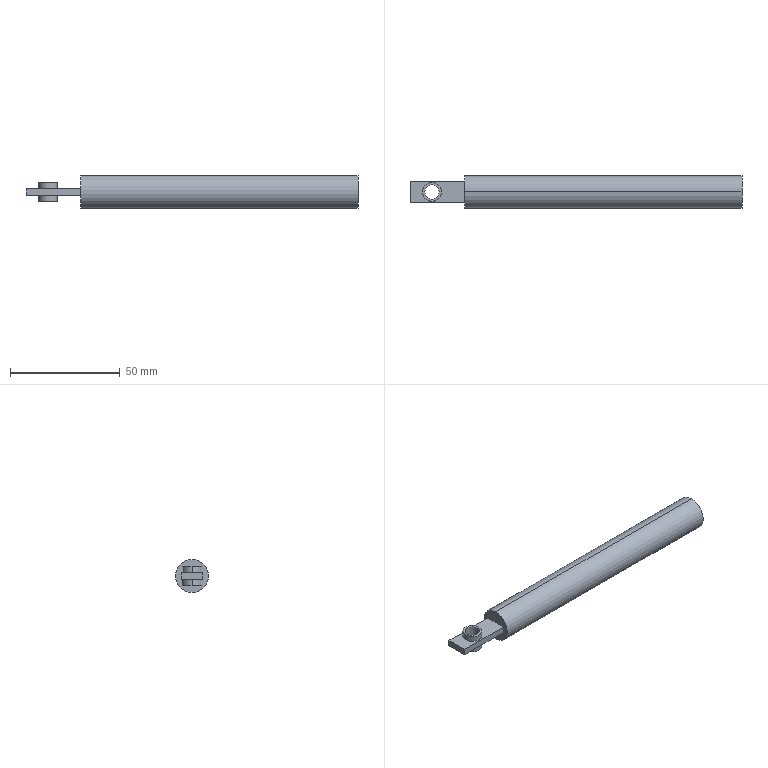Part | STEP file | Gas spring FGS 15089-100 body | 1 solid | 20 faces | box 151 x 15 x 15 mm | volume 18389 mm3 | cylinder 10 | plane 10 | commonest cylinder face diameters 8.5 x4 6.5 x2 7 x2 15 x2
STEP:
#1=CARTESIAN_POINT('',(0.,0.,0.));
#2=DIRECTION('',(0.,0.,1.));
#3=DIRECTION('',(1.,0.,0.));
#4=AXIS2_PLACEMENT_3D('',#1,#2,#3);
#5=CARTESIAN_POINT('',(-11.75,0.,-4.25));
#6=VERTEX_POINT('',#5);
#7=CARTESIAN_POINT('',(-11.75,0.,4.25));
#8=VERTEX_POINT('',#7);
#9=CARTESIAN_POINT('',(-11.75,0.,-4.25));
#10=DIRECTION('',(0.,0.,1.));
#11=VECTOR('',#10,1.);
#12=LINE('',#9,#11);
#13=CARTESIAN_POINT('',(-15.,0.,-4.25));
#14=DIRECTION('',(0.,0.,1.));
#15=DIRECTION('',(1.,0.,0.));
#16=AXIS2_PLACEMENT_3D('',#13,#14,#15);
#17=CYLINDRICAL_SURFACE('',#16,3.25);
#18=CARTESIAN_POINT('',(6.283,0.));
#19=DIRECTION('',(0.,1.));
#20=VECTOR('',#19,1.);
#21=LINE('',#18,#20);
#22=(GEOMETRIC_REPRESENTATION_CONTEXT(2)PARAMETRIC_REPRESENTATION_CONTEXT()REPRESENTATION_CONTEXT('',''));
#23=DEFINITIONAL_REPRESENTATION('',(#21),#22);
#24=PCURVE('',#17,#23);
#25=CARTESIAN_POINT('',(-15.,0.,-4.25));
#26=DIRECTION('',(0.,0.,1.));
#27=DIRECTION('',(1.,0.,0.));
#28=AXIS2_PLACEMENT_3D('',#25,#26,#27);
#29=CYLINDRICAL_SURFACE('',#28,3.25);
#30=CARTESIAN_POINT('',(0.,0.));
#31=DIRECTION('',(0.,1.));
#32=VECTOR('',#31,1.);
#33=LINE('',#30,#32);
#34=(GEOMETRIC_REPRESENTATION_CONTEXT(2)PARAMETRIC_REPRESENTATION_CONTEXT()REPRESENTATION_CONTEXT('',''));
#35=DEFINITIONAL_REPRESENTATION('',(#33),#34);
#36=PCURVE('',#29,#35);
#37=SURFACE_CURVE('',#12,(#24,#36),.PCURVE_S1.);
#38=EDGE_CURVE('',#6,#8,#37,.T.);
#39=ORIENTED_EDGE('',*,*,#38,.T.);
#40=CARTESIAN_POINT('',(-18.25,0.,4.25));
#41=VERTEX_POINT('',#40);
#42=CARTESIAN_POINT('',(-15.,0.,4.25));
#43=DIRECTION('',(0.,0.,1.));
#44=DIRECTION('',(1.,0.,0.));
#45=AXIS2_PLACEMENT_3D('',#42,#43,#44);
#46=CIRCLE('',#45,3.25);
#47=CARTESIAN_POINT('',(0.,8.5));
#48=DIRECTION('',(1.,0.));
#49=VECTOR('',#48,1.);
#50=LINE('',#47,#49);
#51=(GEOMETRIC_REPRESENTATION_CONTEXT(2)PARAMETRIC_REPRESENTATION_CONTEXT()REPRESENTATION_CONTEXT('',''));
#52=DEFINITIONAL_REPRESENTATION('',(#50),#51);
#53=PCURVE('',#17,#52);
#54=CARTESIAN_POINT('',(-19.301,-4.301,4.25));
#55=DIRECTION('',(0.,0.,1.));
#56=DIRECTION('',(1.,0.,0.));
#57=AXIS2_PLACEMENT_3D('',#54,#55,#56);
#58=PLANE('',#57);
#59=CARTESIAN_POINT('',(4.301,4.301));
#60=DIRECTION('',(1.,0.));
#61=AXIS2_PLACEMENT_2D('',#59,#60);
#62=CIRCLE('',#61,3.25);
#63=(GEOMETRIC_REPRESENTATION_CONTEXT(2)PARAMETRIC_REPRESENTATION_CONTEXT()REPRESENTATION_CONTEXT('',''));
#64=DEFINITIONAL_REPRESENTATION('',(#62),#63);
#65=PCURVE('',#58,#64);
#66=SURFACE_CURVE('',#46,(#53,#65),.PCURVE_S1.);
#67=EDGE_CURVE('',#41,#8,#66,.T.);
#68=ORIENTED_EDGE('',*,*,#67,.F.);
#69=CARTESIAN_POINT('',(-18.25,0.,-4.25));
#70=VERTEX_POINT('',#69);
#71=CARTESIAN_POINT('',(-18.25,0.,-4.25));
#72=DIRECTION('',(0.,0.,1.));
#73=VECTOR('',#72,1.);
#74=LINE('',#71,#73);
#75=CARTESIAN_POINT('',(3.142,0.));
#76=DIRECTION('',(0.,1.));
#77=VECTOR('',#76,1.);
#78=LINE('',#75,#77);
#79=(GEOMETRIC_REPRESENTATION_CONTEXT(2)PARAMETRIC_REPRESENTATION_CONTEXT()REPRESENTATION_CONTEXT('',''));
#80=DEFINITIONAL_REPRESENTATION('',(#78),#79);
#81=PCURVE('',#17,#80);
#82=CARTESIAN_POINT('',(3.142,0.));
#83=DIRECTION('',(0.,1.));
#84=VECTOR('',#83,1.);
#85=LINE('',#82,#84);
#86=(GEOMETRIC_REPRESENTATION_CONTEXT(2)PARAMETRIC_REPRESENTATION_CONTEXT()REPRESENTATION_CONTEXT('',''));
#87=DEFINITIONAL_REPRESENTATION('',(#85),#86);
#88=PCURVE('',#29,#87);
#89=SURFACE_CURVE('',#74,(#81,#88),.PCURVE_S1.);
#90=EDGE_CURVE('',#70,#41,#89,.T.);
#91=ORIENTED_EDGE('',*,*,#90,.F.);
#92=CARTESIAN_POINT('',(-15.,0.,-4.25));
#93=DIRECTION('',(0.,0.,-1.));
#94=DIRECTION('',(1.,0.,0.));
#95=AXIS2_PLACEMENT_3D('',#92,#93,#94);
#96=CIRCLE('',#95,3.25);
#97=CARTESIAN_POINT('',(6.283,0.));
#98=DIRECTION('',(-1.,0.));
#99=VECTOR('',#98,1.);
#100=LINE('',#97,#99);
#101=(GEOMETRIC_REPRESENTATION_CONTEXT(2)PARAMETRIC_REPRESENTATION_CONTEXT()REPRESENTATION_CONTEXT('',''));
#102=DEFINITIONAL_REPRESENTATION('',(#100),#101);
#103=PCURVE('',#17,#102);
#104=CARTESIAN_POINT('',(-19.301,-4.301,-4.25));
#105=DIRECTION('',(0.,0.,1.));
#106=DIRECTION('',(1.,0.,0.));
#107=AXIS2_PLACEMENT_3D('',#104,#105,#106);
#108=PLANE('',#107);
#109=CARTESIAN_POINT('',(7.551,4.301));
#110=CARTESIAN_POINT('',(7.551,-1.328));
#111=CARTESIAN_POINT('',(2.676,1.486));
#112=CARTESIAN_POINT('',(-2.199,4.301));
#113=CARTESIAN_POINT('',(2.676,7.116));
#114=CARTESIAN_POINT('',(7.551,9.93));
#115=CARTESIAN_POINT('',(7.551,4.301));
#116=(BOUNDED_CURVE()B_SPLINE_CURVE(2,(#109,#110,#111,#112,#113,#114,#115),.UNSPECIFIED.,.T.,.F.)B_SPLINE_CURVE_WITH_KNOTS((1,2,2,2,2,1),(-2.094,0.,2.094,4.189,6.283,8.378),.UNSPECIFIED.)CURVE()GEOMETRIC_REPRESENTATION_ITEM()RATIONAL_B_SPLINE_CURVE((1.,0.5,1.,0.5,1.,0.5,1.))REPRESENTATION_ITEM(''));
#117=(GEOMETRIC_REPRESENTATION_CONTEXT(2)PARAMETRIC_REPRESENTATION_CONTEXT()REPRESENTATION_CONTEXT('',''));
#118=DEFINITIONAL_REPRESENTATION('',(#116),#117);
#119=PCURVE('',#108,#118);
#120=SURFACE_CURVE('',#96,(#103,#119),.PCURVE_S1.);
#121=EDGE_CURVE('',#6,#70,#120,.T.);
#122=ORIENTED_EDGE('',*,*,#121,.F.);
#123=EDGE_LOOP('',(#39,#68,#91,#122));
#124=FACE_BOUND('',#123,.F.);
#125=ADVANCED_FACE('',(#124),#17,.F.);
#126=CARTESIAN_POINT('',(-10.75,0.,4.25));
#127=VERTEX_POINT('',#126);
#128=CARTESIAN_POINT('',(-19.25,0.,4.25));
#129=VERTEX_POINT('',#128);
#130=CARTESIAN_POINT('',(-15.,0.,4.25));
#131=DIRECTION('',(0.,0.,1.));
#132=DIRECTION('',(-1.,0.,0.));
#133=AXIS2_PLACEMENT_3D('',#130,#131,#132);
#134=CIRCLE('',#133,4.25);
#135=CARTESIAN_POINT('',(-15.,0.,4.25));
#136=DIRECTION('',(0.,0.,-1.));
#137=DIRECTION('',(-1.,0.,0.));
#138=AXIS2_PLACEMENT_3D('',#135,#136,#137);
#139=CYLINDRICAL_SURFACE('',#138,4.25);
#140=CARTESIAN_POINT('',(6.283,0.));
#141=DIRECTION('',(-1.,0.));
#142=VECTOR('',#141,1.);
#143=LINE('',#140,#142);
#144=(GEOMETRIC_REPRESENTATION_CONTEXT(2)PARAMETRIC_REPRESENTATION_CONTEXT()REPRESENTATION_CONTEXT('',''));
#145=DEFINITIONAL_REPRESENTATION('',(#143),#144);
#146=PCURVE('',#139,#145);
#147=CARTESIAN_POINT('',(4.301,4.301));
#148=DIRECTION('',(-1.,0.));
#149=AXIS2_PLACEMENT_2D('',#147,#148);
#150=CIRCLE('',#149,4.25);
#151=(GEOMETRIC_REPRESENTATION_CONTEXT(2)PARAMETRIC_REPRESENTATION_CONTEXT()REPRESENTATION_CONTEXT('',''));
#152=DEFINITIONAL_REPRESENTATION('',(#150),#151);
#153=PCURVE('',#58,#152);
#154=SURFACE_CURVE('',#134,(#146,#153),.PCURVE_S1.);
#155=EDGE_CURVE('',#127,#129,#154,.T.);
#156=ORIENTED_EDGE('',*,*,#155,.F.);
#157=CARTESIAN_POINT('',(-10.75,0.,1.5));
#158=VERTEX_POINT('',#157);
#159=CARTESIAN_POINT('',(-10.75,0.,4.25));
#160=DIRECTION('',(0.,0.,-1.));
#161=VECTOR('',#160,1.);
#162=LINE('',#159,#161);
#163=CARTESIAN_POINT('',(3.142,0.));
#164=DIRECTION('',(0.,1.));
#165=VECTOR('',#164,1.);
#166=LINE('',#163,#165);
#167=(GEOMETRIC_REPRESENTATION_CONTEXT(2)PARAMETRIC_REPRESENTATION_CONTEXT()REPRESENTATION_CONTEXT('',''));
#168=DEFINITIONAL_REPRESENTATION('',(#166),#167);
#169=PCURVE('',#139,#168);
#170=CARTESIAN_POINT('',(-15.,0.,4.25));
#171=DIRECTION('',(0.,0.,-1.));
#172=DIRECTION('',(-1.,0.,0.));
#173=AXIS2_PLACEMENT_3D('',#170,#171,#172);
#174=CYLINDRICAL_SURFACE('',#173,4.25);
#175=CARTESIAN_POINT('',(3.142,0.));
#176=DIRECTION('',(0.,1.));
#177=VECTOR('',#176,1.);
#178=LINE('',#175,#177);
#179=(GEOMETRIC_REPRESENTATION_CONTEXT(2)PARAMETRIC_REPRESENTATION_CONTEXT()REPRESENTATION_CONTEXT('',''));
#180=DEFINITIONAL_REPRESENTATION('',(#178),#179);
#181=PCURVE('',#174,#180);
#182=SURFACE_CURVE('',#162,(#169,#181),.PCURVE_S1.);
#183=EDGE_CURVE('',#127,#158,#182,.T.);
#184=ORIENTED_EDGE('',*,*,#183,.T.);
#185=CARTESIAN_POINT('',(-19.25,0.,1.5));
#186=VERTEX_POINT('',#185);
#187=CARTESIAN_POINT('',(-15.,0.,1.5));
#188=DIRECTION('',(0.,0.,-1.));
#189=DIRECTION('',(-1.,0.,0.));
#190=AXIS2_PLACEMENT_3D('',#187,#188,#189);
#191=CIRCLE('',#190,4.25);
#192=CARTESIAN_POINT('',(0.,2.75));
#193=DIRECTION('',(1.,0.));
#194=VECTOR('',#193,1.);
#195=LINE('',#192,#194);
#196=(GEOMETRIC_REPRESENTATION_CONTEXT(2)PARAMETRIC_REPRESENTATION_CONTEXT()REPRESENTATION_CONTEXT('',''));
#197=DEFINITIONAL_REPRESENTATION('',(#195),#196);
#198=PCURVE('',#139,#197);
#199=CARTESIAN_POINT('',(0.,-5.,1.5));
#200=DIRECTION('',(0.,0.,-1.));
#201=DIRECTION('',(-1.,0.,0.));
#202=AXIS2_PLACEMENT_3D('',#199,#200,#201);
#203=PLANE('',#202);
#204=CARTESIAN_POINT('',(15.,5.));
#205=DIRECTION('',(1.,0.));
#206=AXIS2_PLACEMENT_2D('',#204,#205);
#207=CIRCLE('',#206,4.25);
#208=(GEOMETRIC_REPRESENTATION_CONTEXT(2)PARAMETRIC_REPRESENTATION_CONTEXT()REPRESENTATION_CONTEXT('',''));
#209=DEFINITIONAL_REPRESENTATION('',(#207),#208);
#210=PCURVE('',#203,#209);
#211=SURFACE_CURVE('',#191,(#198,#210),.PCURVE_S1.);
#212=EDGE_CURVE('',#186,#158,#211,.T.);
#213=ORIENTED_EDGE('',*,*,#212,.F.);
#214=CARTESIAN_POINT('',(-19.25,0.,4.25));
#215=DIRECTION('',(0.,0.,-1.));
#216=VECTOR('',#215,1.);
#217=LINE('',#214,#216);
#218=CARTESIAN_POINT('',(0.,0.));
#219=DIRECTION('',(0.,1.));
#220=VECTOR('',#219,1.);
#221=LINE('',#218,#220);
#222=(GEOMETRIC_REPRESENTATION_CONTEXT(2)PARAMETRIC_REPRESENTATION_CONTEXT()REPRESENTATION_CONTEXT('',''));
#223=DEFINITIONAL_REPRESENTATION('',(#221),#222);
#224=PCURVE('',#139,#223);
#225=CARTESIAN_POINT('',(6.283,0.));
#226=DIRECTION('',(0.,1.));
#227=VECTOR('',#226,1.);
#228=LINE('',#225,#227);
#229=(GEOMETRIC_REPRESENTATION_CONTEXT(2)PARAMETRIC_REPRESENTATION_CONTEXT()REPRESENTATION_CONTEXT('',''));
#230=DEFINITIONAL_REPRESENTATION('',(#228),#229);
#231=PCURVE('',#174,#230);
#232=SURFACE_CURVE('',#217,(#224,#231),.PCURVE_S1.);
#233=EDGE_CURVE('',#129,#186,#232,.T.);
#234=ORIENTED_EDGE('',*,*,#233,.F.);
#235=EDGE_LOOP('',(#156,#184,#213,#234));
#236=FACE_BOUND('',#235,.T.);
#237=ADVANCED_FACE('',(#236),#139,.T.);
#238=CARTESIAN_POINT('',(-10.75,0.,-1.5));
#239=VERTEX_POINT('',#238);
#240=CARTESIAN_POINT('',(-19.25,0.,-1.5));
#241=VERTEX_POINT('',#240);
#242=CARTESIAN_POINT('',(-15.,0.,-1.5));
#243=DIRECTION('',(0.,0.,1.));
#244=DIRECTION('',(-1.,0.,0.));
#245=AXIS2_PLACEMENT_3D('',#242,#243,#244);
#246=CIRCLE('',#245,4.25);
#247=CARTESIAN_POINT('',(-15.,0.,-1.5));
#248=DIRECTION('',(0.,0.,-1.));
#249=DIRECTION('',(-1.,0.,0.));
#250=AXIS2_PLACEMENT_3D('',#247,#248,#249);
#251=CYLINDRICAL_SURFACE('',#250,4.25);
#252=CARTESIAN_POINT('',(6.283,0.));
#253=DIRECTION('',(-1.,0.));
#254=VECTOR('',#253,1.);
#255=LINE('',#252,#254);
#256=(GEOMETRIC_REPRESENTATION_CONTEXT(2)PARAMETRIC_REPRESENTATION_CONTEXT()REPRESENTATION_CONTEXT('',''));
#257=DEFINITIONAL_REPRESENTATION('',(#255),#256);
#258=PCURVE('',#251,#257);
#259=CARTESIAN_POINT('',(-25.,-5.,-1.5));
#260=DIRECTION('',(0.,0.,1.));
#261=DIRECTION('',(1.,0.,0.));
#262=AXIS2_PLACEMENT_3D('',#259,#260,#261);
#263=PLANE('',#262);
#264=CARTESIAN_POINT('',(10.,5.));
#265=DIRECTION('',(-1.,0.));
#266=AXIS2_PLACEMENT_2D('',#264,#265);
#267=CIRCLE('',#266,4.25);
#268=(GEOMETRIC_REPRESENTATION_CONTEXT(2)PARAMETRIC_REPRESENTATION_CONTEXT()REPRESENTATION_CONTEXT('',''));
#269=DEFINITIONAL_REPRESENTATION('',(#267),#268);
#270=PCURVE('',#263,#269);
#271=SURFACE_CURVE('',#246,(#258,#270),.PCURVE_S1.);
#272=EDGE_CURVE('',#239,#241,#271,.T.);
#273=ORIENTED_EDGE('',*,*,#272,.F.);
#274=CARTESIAN_POINT('',(-10.75,0.,-4.25));
#275=VERTEX_POINT('',#274);
#276=CARTESIAN_POINT('',(-10.75,0.,-1.5));
#277=DIRECTION('',(0.,0.,-1.));
#278=VECTOR('',#277,1.);
#279=LINE('',#276,#278);
#280=CARTESIAN_POINT('',(3.142,0.));
#281=DIRECTION('',(0.,1.));
#282=VECTOR('',#281,1.);
#283=LINE('',#280,#282);
#284=(GEOMETRIC_REPRESENTATION_CONTEXT(2)PARAMETRIC_REPRESENTATION_CONTEXT()REPRESENTATION_CONTEXT('',''));
#285=DEFINITIONAL_REPRESENTATION('',(#283),#284);
#286=PCURVE('',#251,#285);
#287=CARTESIAN_POINT('',(-15.,0.,-1.5));
#288=DIRECTION('',(0.,0.,-1.));
#289=DIRECTION('',(-1.,0.,0.));
#290=AXIS2_PLACEMENT_3D('',#287,#288,#289);
#291=CYLINDRICAL_SURFACE('',#290,4.25);
#292=CARTESIAN_POINT('',(3.142,0.));
#293=DIRECTION('',(0.,1.));
#294=VECTOR('',#293,1.);
#295=LINE('',#292,#294);
#296=(GEOMETRIC_REPRESENTATION_CONTEXT(2)PARAMETRIC_REPRESENTATION_CONTEXT()REPRESENTATION_CONTEXT('',''));
#297=DEFINITIONAL_REPRESENTATION('',(#295),#296);
#298=PCURVE('',#291,#297);
#299=SURFACE_CURVE('',#279,(#286,#298),.PCURVE_S1.);
#300=EDGE_CURVE('',#239,#275,#299,.T.);
#301=ORIENTED_EDGE('',*,*,#300,.T.);
#302=CARTESIAN_POINT('',(-19.25,0.,-4.25));
#303=VERTEX_POINT('',#302);
#304=CARTESIAN_POINT('',(-15.,0.,-4.25));
#305=DIRECTION('',(0.,0.,1.));
#306=DIRECTION('',(-1.,0.,0.));
#307=AXIS2_PLACEMENT_3D('',#304,#305,#306);
#308=CIRCLE('',#307,4.25);
#309=CARTESIAN_POINT('',(6.283,2.75));
#310=DIRECTION('',(-1.,0.));
#311=VECTOR('',#310,1.);
#312=LINE('',#309,#311);
#313=(GEOMETRIC_REPRESENTATION_CONTEXT(2)PARAMETRIC_REPRESENTATION_CONTEXT()REPRESENTATION_CONTEXT('',''));
#314=DEFINITIONAL_REPRESENTATION('',(#312),#313);
#315=PCURVE('',#251,#314);
#316=CARTESIAN_POINT('',(4.301,4.301));
#317=DIRECTION('',(-1.,0.));
#318=AXIS2_PLACEMENT_2D('',#316,#317);
#319=CIRCLE('',#318,4.25);
#320=(GEOMETRIC_REPRESENTATION_CONTEXT(2)PARAMETRIC_REPRESENTATION_CONTEXT()REPRESENTATION_CONTEXT('',''));
#321=DEFINITIONAL_REPRESENTATION('',(#319),#320);
#322=PCURVE('',#108,#321);
#323=SURFACE_CURVE('',#308,(#315,#322),.PCURVE_S1.);
#324=EDGE_CURVE('',#275,#303,#323,.T.);
#325=ORIENTED_EDGE('',*,*,#324,.T.);
#326=CARTESIAN_POINT('',(-19.25,0.,-1.5));
#327=DIRECTION('',(0.,0.,-1.));
#328=VECTOR('',#327,1.);
#329=LINE('',#326,#328);
#330=CARTESIAN_POINT('',(0.,0.));
#331=DIRECTION('',(0.,1.));
#332=VECTOR('',#331,1.);
#333=LINE('',#330,#332);
#334=(GEOMETRIC_REPRESENTATION_CONTEXT(2)PARAMETRIC_REPRESENTATION_CONTEXT()REPRESENTATION_CONTEXT('',''));
#335=DEFINITIONAL_REPRESENTATION('',(#333),#334);
#336=PCURVE('',#251,#335);
#337=CARTESIAN_POINT('',(6.283,0.));
#338=DIRECTION('',(0.,1.));
#339=VECTOR('',#338,1.);
#340=LINE('',#337,#339);
#341=(GEOMETRIC_REPRESENTATION_CONTEXT(2)PARAMETRIC_REPRESENTATION_CONTEXT()REPRESENTATION_CONTEXT('',''));
#342=DEFINITIONAL_REPRESENTATION('',(#340),#341);
#343=PCURVE('',#291,#342);
#344=SURFACE_CURVE('',#329,(#336,#343),.PCURVE_S1.);
#345=EDGE_CURVE('',#241,#303,#344,.T.);
#346=ORIENTED_EDGE('',*,*,#345,.F.);
#347=EDGE_LOOP('',(#273,#301,#325,#346));
#348=FACE_BOUND('',#347,.T.);
#349=ADVANCED_FACE('',(#348),#251,.T.);
#350=CARTESIAN_POINT('',(126.,0.,-7.5));
#351=VERTEX_POINT('',#350);
#352=CARTESIAN_POINT('',(126.,0.,7.5));
#353=VERTEX_POINT('',#352);
#354=CARTESIAN_POINT('',(126.,0.,0.));
#355=DIRECTION('',(1.,0.,0.));
#356=DIRECTION('',(0.,0.,1.));
#357=AXIS2_PLACEMENT_3D('',#354,#355,#356);
#358=CIRCLE('',#357,7.5);
#359=CARTESIAN_POINT('',(126.,0.,0.));
#360=DIRECTION('',(-1.,0.,0.));
#361=DIRECTION('',(0.,0.,1.));
#362=AXIS2_PLACEMENT_3D('',#359,#360,#361);
#363=CYLINDRICAL_SURFACE('',#362,7.5);
#364=CARTESIAN_POINT('',(6.283,0.));
#365=DIRECTION('',(-1.,0.));
#366=VECTOR('',#365,1.);
#367=LINE('',#364,#366);
#368=(GEOMETRIC_REPRESENTATION_CONTEXT(2)PARAMETRIC_REPRESENTATION_CONTEXT()REPRESENTATION_CONTEXT('',''));
#369=DEFINITIONAL_REPRESENTATION('',(#367),#368);
#370=PCURVE('',#363,#369);
#371=CARTESIAN_POINT('',(126.,-7.59,7.59));
#372=DIRECTION('',(1.,0.,0.));
#373=DIRECTION('',(0.,0.,-1.));
#374=AXIS2_PLACEMENT_3D('',#371,#372,#373);
#375=PLANE('',#374);
#376=CARTESIAN_POINT('',(7.59,7.59));
#377=DIRECTION('',(-1.,0.));
#378=AXIS2_PLACEMENT_2D('',#376,#377);
#379=CIRCLE('',#378,7.5);
#380=(GEOMETRIC_REPRESENTATION_CONTEXT(2)PARAMETRIC_REPRESENTATION_CONTEXT()REPRESENTATION_CONTEXT('',''));
#381=DEFINITIONAL_REPRESENTATION('',(#379),#380);
#382=PCURVE('',#375,#381);
#383=SURFACE_CURVE('',#358,(#370,#382),.PCURVE_S1.);
#384=EDGE_CURVE('',#351,#353,#383,.T.);
#385=ORIENTED_EDGE('',*,*,#384,.F.);
#386=CARTESIAN_POINT('',(0.,0.,-7.5));
#387=VERTEX_POINT('',#386);
#388=CARTESIAN_POINT('',(126.,0.,-7.5));
#389=DIRECTION('',(-1.,0.,0.));
#390=VECTOR('',#389,1.);
#391=LINE('',#388,#390);
#392=CARTESIAN_POINT('',(3.142,0.));
#393=DIRECTION('',(0.,1.));
#394=VECTOR('',#393,1.);
#395=LINE('',#392,#394);
#396=(GEOMETRIC_REPRESENTATION_CONTEXT(2)PARAMETRIC_REPRESENTATION_CONTEXT()REPRESENTATION_CONTEXT('',''));
#397=DEFINITIONAL_REPRESENTATION('',(#395),#396);
#398=PCURVE('',#363,#397);
#399=CARTESIAN_POINT('',(126.,0.,0.));
#400=DIRECTION('',(-1.,0.,0.));
#401=DIRECTION('',(0.,0.,1.));
#402=AXIS2_PLACEMENT_3D('',#399,#400,#401);
#403=CYLINDRICAL_SURFACE('',#402,7.5);
#404=CARTESIAN_POINT('',(3.142,0.));
#405=DIRECTION('',(0.,1.));
#406=VECTOR('',#405,1.);
#407=LINE('',#404,#406);
#408=(GEOMETRIC_REPRESENTATION_CONTEXT(2)PARAMETRIC_REPRESENTATION_CONTEXT()REPRESENTATION_CONTEXT('',''));
#409=DEFINITIONAL_REPRESENTATION('',(#407),#408);
#410=PCURVE('',#403,#409);
#411=SURFACE_CURVE('',#391,(#398,#410),.PCURVE_S1.);
#412=EDGE_CURVE('',#351,#387,#411,.T.);
#413=ORIENTED_EDGE('',*,*,#412,.T.);
#414=CARTESIAN_POINT('',(0.,0.,7.5));
#415=VERTEX_POINT('',#414);
#416=CARTESIAN_POINT('',(0.,0.,0.));
#417=DIRECTION('',(1.,0.,0.));
#418=DIRECTION('',(0.,0.,1.));
#419=AXIS2_PLACEMENT_3D('',#416,#417,#418);
#420=CIRCLE('',#419,7.5);
#421=CARTESIAN_POINT('',(6.283,126.));
#422=DIRECTION('',(-1.,0.));
#423=VECTOR('',#422,1.);
#424=LINE('',#421,#423);
#425=(GEOMETRIC_REPRESENTATION_CONTEXT(2)PARAMETRIC_REPRESENTATION_CONTEXT()REPRESENTATION_CONTEXT('',''));
#426=DEFINITIONAL_REPRESENTATION('',(#424),#425);
#427=PCURVE('',#363,#426);
#428=CARTESIAN_POINT('',(0.,-7.59,7.59));
#429=DIRECTION('',(1.,0.,0.));
#430=DIRECTION('',(0.,0.,-1.));
#431=AXIS2_PLACEMENT_3D('',#428,#429,#430);
#432=PLANE('',#431);
#433=CARTESIAN_POINT('',(7.59,7.59));
#434=DIRECTION('',(-1.,0.));
#435=AXIS2_PLACEMENT_2D('',#433,#434);
#436=CIRCLE('',#435,7.5);
#437=(GEOMETRIC_REPRESENTATION_CONTEXT(2)PARAMETRIC_REPRESENTATION_CONTEXT()REPRESENTATION_CONTEXT('',''));
#438=DEFINITIONAL_REPRESENTATION('',(#436),#437);
#439=PCURVE('',#432,#438);
#440=SURFACE_CURVE('',#420,(#427,#439),.PCURVE_S1.);
#441=EDGE_CURVE('',#387,#415,#440,.T.);
#442=ORIENTED_EDGE('',*,*,#441,.T.);
#443=CARTESIAN_POINT('',(126.,0.,7.5));
#444=DIRECTION('',(-1.,0.,0.));
#445=VECTOR('',#444,1.);
#446=LINE('',#443,#445);
#447=CARTESIAN_POINT('',(0.,0.));
#448=DIRECTION('',(0.,1.));
#449=VECTOR('',#448,1.);
#450=LINE('',#447,#449);
#451=(GEOMETRIC_REPRESENTATION_CONTEXT(2)PARAMETRIC_REPRESENTATION_CONTEXT()REPRESENTATION_CONTEXT('',''));
#452=DEFINITIONAL_REPRESENTATION('',(#450),#451);
#453=PCURVE('',#363,#452);
#454=CARTESIAN_POINT('',(6.283,0.));
#455=DIRECTION('',(0.,1.));
#456=VECTOR('',#455,1.);
#457=LINE('',#454,#456);
#458=(GEOMETRIC_REPRESENTATION_CONTEXT(2)PARAMETRIC_REPRESENTATION_CONTEXT()REPRESENTATION_CONTEXT('',''));
#459=DEFINITIONAL_REPRESENTATION('',(#457),#458);
#460=PCURVE('',#403,#459);
#461=SURFACE_CURVE('',#446,(#453,#460),.PCURVE_S1.);
#462=EDGE_CURVE('',#353,#415,#461,.T.);
#463=ORIENTED_EDGE('',*,*,#462,.F.);
#464=EDGE_LOOP('',(#385,#413,#442,#463));
#465=FACE_BOUND('',#464,.T.);
#466=ADVANCED_FACE('',(#465),#363,.T.);
#467=CARTESIAN_POINT('',(126.,0.,3.5));
#468=VERTEX_POINT('',#467);
#469=CARTESIAN_POINT('',(5.,0.,3.5));
#470=VERTEX_POINT('',#469);
#471=CARTESIAN_POINT('',(126.,0.,3.5));
#472=DIRECTION('',(-1.,0.,0.));
#473=VECTOR('',#472,1.);
#474=LINE('',#471,#473);
#475=CARTESIAN_POINT('',(126.,0.,0.));
#476=DIRECTION('',(-1.,0.,0.));
#477=DIRECTION('',(0.,0.,1.));
#478=AXIS2_PLACEMENT_3D('',#475,#476,#477);
#479=CYLINDRICAL_SURFACE('',#478,3.5);
#480=CARTESIAN_POINT('',(6.283,0.));
#481=DIRECTION('',(0.,1.));
#482=VECTOR('',#481,1.);
#483=LINE('',#480,#482);
#484=(GEOMETRIC_REPRESENTATION_CONTEXT(2)PARAMETRIC_REPRESENTATION_CONTEXT()REPRESENTATION_CONTEXT('',''));
#485=DEFINITIONAL_REPRESENTATION('',(#483),#484);
#486=PCURVE('',#479,#485);
#487=CARTESIAN_POINT('',(126.,0.,0.));
#488=DIRECTION('',(-1.,0.,0.));
#489=DIRECTION('',(0.,0.,1.));
#490=AXIS2_PLACEMENT_3D('',#487,#488,#489);
#491=CYLINDRICAL_SURFACE('',#490,3.5);
#492=CARTESIAN_POINT('',(0.,0.));
#493=DIRECTION('',(0.,1.));
#494=VECTOR('',#493,1.);
#495=LINE('',#492,#494);
#496=(GEOMETRIC_REPRESENTATION_CONTEXT(2)PARAMETRIC_REPRESENTATION_CONTEXT()REPRESENTATION_CONTEXT('',''));
#497=DEFINITIONAL_REPRESENTATION('',(#495),#496);
#498=PCURVE('',#491,#497);
#499=SURFACE_CURVE('',#474,(#486,#498),.PCURVE_S1.);
#500=EDGE_CURVE('',#468,#470,#499,.T.);
#501=ORIENTED_EDGE('',*,*,#500,.T.);
#502=CARTESIAN_POINT('',(5.,0.,-3.5));
#503=VERTEX_POINT('',#502);
#504=CARTESIAN_POINT('',(5.,0.,0.));
#505=DIRECTION('',(-1.,0.,0.));
#506=DIRECTION('',(0.,0.,1.));
#507=AXIS2_PLACEMENT_3D('',#504,#505,#506);
#508=CIRCLE('',#507,3.5);
#509=CARTESIAN_POINT('',(0.,121.));
#510=DIRECTION('',(1.,0.));
#511=VECTOR('',#510,1.);
#512=LINE('',#509,#511);
#513=(GEOMETRIC_REPRESENTATION_CONTEXT(2)PARAMETRIC_REPRESENTATION_CONTEXT()REPRESENTATION_CONTEXT('',''));
#514=DEFINITIONAL_REPRESENTATION('',(#512),#513);
#515=PCURVE('',#479,#514);
#516=CARTESIAN_POINT('',(5.,-3.542,-3.542));
#517=DIRECTION('',(-1.,0.,0.));
#518=DIRECTION('',(0.,0.,1.));
#519=AXIS2_PLACEMENT_3D('',#516,#517,#518);
#520=PLANE('',#519);
#521=CARTESIAN_POINT('',(3.542,3.542));
#522=DIRECTION('',(1.,0.));
#523=AXIS2_PLACEMENT_2D('',#521,#522);
#524=CIRCLE('',#523,3.5);
#525=(GEOMETRIC_REPRESENTATION_CONTEXT(2)PARAMETRIC_REPRESENTATION_CONTEXT()REPRESENTATION_CONTEXT('',''));
#526=DEFINITIONAL_REPRESENTATION('',(#524),#525);
#527=PCURVE('',#520,#526);
#528=SURFACE_CURVE('',#508,(#515,#527),.PCURVE_S1.);
#529=EDGE_CURVE('',#503,#470,#528,.T.);
#530=ORIENTED_EDGE('',*,*,#529,.F.);
#531=CARTESIAN_POINT('',(126.,0.,-3.5));
#532=VERTEX_POINT('',#531);
#533=CARTESIAN_POINT('',(126.,0.,-3.5));
#534=DIRECTION('',(-1.,0.,0.));
#535=VECTOR('',#534,1.);
#536=LINE('',#533,#535);
#537=CARTESIAN_POINT('',(3.142,0.));
#538=DIRECTION('',(0.,1.));
#539=VECTOR('',#538,1.);
#540=LINE('',#537,#539);
#541=(GEOMETRIC_REPRESENTATION_CONTEXT(2)PARAMETRIC_REPRESENTATION_CONTEXT()REPRESENTATION_CONTEXT('',''));
#542=DEFINITIONAL_REPRESENTATION('',(#540),#541);
#543=PCURVE('',#479,#542);
#544=CARTESIAN_POINT('',(3.142,0.));
#545=DIRECTION('',(0.,1.));
#546=VECTOR('',#545,1.);
#547=LINE('',#544,#546);
#548=(GEOMETRIC_REPRESENTATION_CONTEXT(2)PARAMETRIC_REPRESENTATION_CONTEXT()REPRESENTATION_CONTEXT('',''));
#549=DEFINITIONAL_REPRESENTATION('',(#547),#548);
#550=PCURVE('',#491,#549);
#551=SURFACE_CURVE('',#536,(#543,#550),.PCURVE_S1.);
#552=EDGE_CURVE('',#532,#503,#551,.T.);
#553=ORIENTED_EDGE('',*,*,#552,.F.);
#554=CARTESIAN_POINT('',(126.,0.,0.));
#555=DIRECTION('',(-1.,0.,0.));
#556=DIRECTION('',(0.,0.,1.));
#557=AXIS2_PLACEMENT_3D('',#554,#555,#556);
#558=CIRCLE('',#557,3.5);
#559=CARTESIAN_POINT('',(0.,0.));
#560=DIRECTION('',(1.,0.));
#561=VECTOR('',#560,1.);
#562=LINE('',#559,#561);
#563=(GEOMETRIC_REPRESENTATION_CONTEXT(2)PARAMETRIC_REPRESENTATION_CONTEXT()REPRESENTATION_CONTEXT('',''));
#564=DEFINITIONAL_REPRESENTATION('',(#562),#563);
#565=PCURVE('',#479,#564);
#566=CARTESIAN_POINT('',(4.09,7.59));
#567=CARTESIAN_POINT('',(4.09,13.652));
#568=CARTESIAN_POINT('',(9.34,10.621));
#569=CARTESIAN_POINT('',(14.59,7.59));
#570=CARTESIAN_POINT('',(9.34,4.559));
#571=CARTESIAN_POINT('',(4.09,1.528));
#572=CARTESIAN_POINT('',(4.09,7.59));
#573=(BOUNDED_CURVE()B_SPLINE_CURVE(2,(#566,#567,#568,#569,#570,#571,#572),.UNSPECIFIED.,.T.,.F.)B_SPLINE_CURVE_WITH_KNOTS((1,2,2,2,2,1),(-2.094,0.,2.094,4.189,6.283,8.378),.UNSPECIFIED.)CURVE()GEOMETRIC_REPRESENTATION_ITEM()RATIONAL_B_SPLINE_CURVE((1.,0.5,1.,0.5,1.,0.5,1.))REPRESENTATION_ITEM(''));
#574=(GEOMETRIC_REPRESENTATION_CONTEXT(2)PARAMETRIC_REPRESENTATION_CONTEXT()REPRESENTATION_CONTEXT('',''));
#575=DEFINITIONAL_REPRESENTATION('',(#573),#574);
#576=PCURVE('',#375,#575);
#577=SURFACE_CURVE('',#558,(#565,#576),.PCURVE_S1.);
#578=EDGE_CURVE('',#532,#468,#577,.T.);
#579=ORIENTED_EDGE('',*,*,#578,.T.);
#580=EDGE_LOOP('',(#501,#530,#553,#579));
#581=FACE_BOUND('',#580,.F.);
#582=ADVANCED_FACE('',(#581),#479,.F.);
#583=CARTESIAN_POINT('',(-15.,0.,4.25));
#584=DIRECTION('',(0.,0.,1.));
#585=DIRECTION('',(1.,0.,0.));
#586=AXIS2_PLACEMENT_3D('',#583,#584,#585);
#587=CIRCLE('',#586,3.25);
#588=CARTESIAN_POINT('',(0.,8.5));
#589=DIRECTION('',(1.,0.));
#590=VECTOR('',#589,1.);
#591=LINE('',#588,#590);
#592=(GEOMETRIC_REPRESENTATION_CONTEXT(2)PARAMETRIC_REPRESENTATION_CONTEXT()REPRESENTATION_CONTEXT('',''));
#593=DEFINITIONAL_REPRESENTATION('',(#591),#592);
#594=PCURVE('',#29,#593);
#595=CARTESIAN_POINT('',(4.301,4.301));
#596=DIRECTION('',(1.,0.));
#597=AXIS2_PLACEMENT_2D('',#595,#596);
#598=CIRCLE('',#597,3.25);
#599=(GEOMETRIC_REPRESENTATION_CONTEXT(2)PARAMETRIC_REPRESENTATION_CONTEXT()REPRESENTATION_CONTEXT('',''));
#600=DEFINITIONAL_REPRESENTATION('',(#598),#599);
#601=PCURVE('',#58,#600);
#602=SURFACE_CURVE('',#587,(#594,#601),.PCURVE_S1.);
#603=EDGE_CURVE('',#8,#41,#602,.T.);
#604=ORIENTED_EDGE('',*,*,#603,.F.);
#605=ORIENTED_EDGE('',*,*,#38,.F.);
#606=CARTESIAN_POINT('',(-15.,0.,-4.25));
#607=DIRECTION('',(0.,0.,-1.));
#608=DIRECTION('',(1.,0.,0.));
#609=AXIS2_PLACEMENT_3D('',#606,#607,#608);
#610=CIRCLE('',#609,3.25);
#611=CARTESIAN_POINT('',(6.283,0.));
#612=DIRECTION('',(-1.,0.));
#613=VECTOR('',#612,1.);
#614=LINE('',#611,#613);
#615=(GEOMETRIC_REPRESENTATION_CONTEXT(2)PARAMETRIC_REPRESENTATION_CONTEXT()REPRESENTATION_CONTEXT('',''));
#616=DEFINITIONAL_REPRESENTATION('',(#614),#615);
#617=PCURVE('',#29,#616);
#618=CARTESIAN_POINT('',(7.551,4.301));
#619=CARTESIAN_POINT('',(7.551,-1.328));
#620=CARTESIAN_POINT('',(2.676,1.486));
#621=CARTESIAN_POINT('',(-2.199,4.301));
#622=CARTESIAN_POINT('',(2.676,7.116));
#623=CARTESIAN_POINT('',(7.551,9.93));
#624=CARTESIAN_POINT('',(7.551,4.301));
#625=(BOUNDED_CURVE()B_SPLINE_CURVE(2,(#618,#619,#620,#621,#622,#623,#624),.UNSPECIFIED.,.T.,.F.)B_SPLINE_CURVE_WITH_KNOTS((1,2,2,2,2,1),(-2.094,0.,2.094,4.189,6.283,8.378),.UNSPECIFIED.)CURVE()GEOMETRIC_REPRESENTATION_ITEM()RATIONAL_B_SPLINE_CURVE((1.,0.5,1.,0.5,1.,0.5,1.))REPRESENTATION_ITEM(''));
#626=(GEOMETRIC_REPRESENTATION_CONTEXT(2)PARAMETRIC_REPRESENTATION_CONTEXT()REPRESENTATION_CONTEXT('',''));
#627=DEFINITIONAL_REPRESENTATION('',(#625),#626);
#628=PCURVE('',#108,#627);
#629=SURFACE_CURVE('',#610,(#617,#628),.PCURVE_S1.);
#630=EDGE_CURVE('',#70,#6,#629,.T.);
#631=ORIENTED_EDGE('',*,*,#630,.F.);
#632=ORIENTED_EDGE('',*,*,#90,.T.);
#633=EDGE_LOOP('',(#604,#605,#631,#632));
#634=FACE_BOUND('',#633,.F.);
#635=ADVANCED_FACE('',(#634),#29,.F.);
#636=ORIENTED_EDGE('',*,*,#603,.F.);
#637=ORIENTED_EDGE('',*,*,#67,.F.);
#638=EDGE_LOOP('',(#636,#637));
#639=FACE_BOUND('',#638,.T.);
#640=CARTESIAN_POINT('',(-15.,0.,4.25));
#641=DIRECTION('',(0.,0.,1.));
#642=DIRECTION('',(-1.,0.,0.));
#643=AXIS2_PLACEMENT_3D('',#640,#641,#642);
#644=CIRCLE('',#643,4.25);
#645=CARTESIAN_POINT('',(4.301,4.301));
#646=DIRECTION('',(-1.,0.));
#647=AXIS2_PLACEMENT_2D('',#645,#646);
#648=CIRCLE('',#647,4.25);
#649=(GEOMETRIC_REPRESENTATION_CONTEXT(2)PARAMETRIC_REPRESENTATION_CONTEXT()REPRESENTATION_CONTEXT('',''));
#650=DEFINITIONAL_REPRESENTATION('',(#648),#649);
#651=PCURVE('',#58,#650);
#652=CARTESIAN_POINT('',(6.283,0.));
#653=DIRECTION('',(-1.,0.));
#654=VECTOR('',#653,1.);
#655=LINE('',#652,#654);
#656=(GEOMETRIC_REPRESENTATION_CONTEXT(2)PARAMETRIC_REPRESENTATION_CONTEXT()REPRESENTATION_CONTEXT('',''));
#657=DEFINITIONAL_REPRESENTATION('',(#655),#656);
#658=PCURVE('',#174,#657);
#659=SURFACE_CURVE('',#644,(#651,#658),.PCURVE_S1.);
#660=EDGE_CURVE('',#129,#127,#659,.T.);
#661=ORIENTED_EDGE('',*,*,#660,.T.);
#662=ORIENTED_EDGE('',*,*,#155,.T.);
#663=EDGE_LOOP('',(#661,#662));
#664=FACE_BOUND('',#663,.T.);
#665=ADVANCED_FACE('',(#639,#664),#58,.T.);
#666=ORIENTED_EDGE('',*,*,#121,.F.);
#667=ORIENTED_EDGE('',*,*,#630,.F.);
#668=EDGE_LOOP('',(#666,#667));
#669=FACE_BOUND('',#668,.T.);
#670=CARTESIAN_POINT('',(-15.,0.,-4.25));
#671=DIRECTION('',(0.,0.,1.));
#672=DIRECTION('',(-1.,0.,0.));
#673=AXIS2_PLACEMENT_3D('',#670,#671,#672);
#674=CIRCLE('',#673,4.25);
#675=CARTESIAN_POINT('',(4.301,4.301));
#676=DIRECTION('',(-1.,0.));
#677=AXIS2_PLACEMENT_2D('',#675,#676);
#678=CIRCLE('',#677,4.25);
#679=(GEOMETRIC_REPRESENTATION_CONTEXT(2)PARAMETRIC_REPRESENTATION_CONTEXT()REPRESENTATION_CONTEXT('',''));
#680=DEFINITIONAL_REPRESENTATION('',(#678),#679);
#681=PCURVE('',#108,#680);
#682=CARTESIAN_POINT('',(6.283,2.75));
#683=DIRECTION('',(-1.,0.));
#684=VECTOR('',#683,1.);
#685=LINE('',#682,#684);
#686=(GEOMETRIC_REPRESENTATION_CONTEXT(2)PARAMETRIC_REPRESENTATION_CONTEXT()REPRESENTATION_CONTEXT('',''));
#687=DEFINITIONAL_REPRESENTATION('',(#685),#686);
#688=PCURVE('',#291,#687);
#689=SURFACE_CURVE('',#674,(#681,#688),.PCURVE_S1.);
#690=EDGE_CURVE('',#303,#275,#689,.T.);
#691=ORIENTED_EDGE('',*,*,#690,.F.);
#692=ORIENTED_EDGE('',*,*,#324,.F.);
#693=EDGE_LOOP('',(#691,#692));
#694=FACE_BOUND('',#693,.T.);
#695=ADVANCED_FACE('',(#669,#694),#108,.F.);
#696=ORIENTED_EDGE('',*,*,#183,.F.);
#697=ORIENTED_EDGE('',*,*,#660,.F.);
#698=ORIENTED_EDGE('',*,*,#233,.T.);
#699=CARTESIAN_POINT('',(-15.,0.,1.5));
#700=DIRECTION('',(0.,0.,-1.));
#701=DIRECTION('',(-1.,0.,0.));
#702=AXIS2_PLACEMENT_3D('',#699,#700,#701);
#703=CIRCLE('',#702,4.25);
#704=CARTESIAN_POINT('',(0.,2.75));
#705=DIRECTION('',(1.,0.));
#706=VECTOR('',#705,1.);
#707=LINE('',#704,#706);
#708=(GEOMETRIC_REPRESENTATION_CONTEXT(2)PARAMETRIC_REPRESENTATION_CONTEXT()REPRESENTATION_CONTEXT('',''));
#709=DEFINITIONAL_REPRESENTATION('',(#707),#708);
#710=PCURVE('',#174,#709);
#711=CARTESIAN_POINT('',(15.,5.));
#712=DIRECTION('',(1.,0.));
#713=AXIS2_PLACEMENT_2D('',#711,#712);
#714=CIRCLE('',#713,4.25);
#715=(GEOMETRIC_REPRESENTATION_CONTEXT(2)PARAMETRIC_REPRESENTATION_CONTEXT()REPRESENTATION_CONTEXT('',''));
#716=DEFINITIONAL_REPRESENTATION('',(#714),#715);
#717=PCURVE('',#203,#716);
#718=SURFACE_CURVE('',#703,(#710,#717),.PCURVE_S1.);
#719=EDGE_CURVE('',#158,#186,#718,.T.);
#720=ORIENTED_EDGE('',*,*,#719,.F.);
#721=EDGE_LOOP('',(#696,#697,#698,#720));
#722=FACE_BOUND('',#721,.T.);
#723=ADVANCED_FACE('',(#722),#174,.T.);
#724=ORIENTED_EDGE('',*,*,#300,.F.);
#725=CARTESIAN_POINT('',(-15.,0.,-1.5));
#726=DIRECTION('',(0.,0.,1.));
#727=DIRECTION('',(-1.,0.,0.));
#728=AXIS2_PLACEMENT_3D('',#725,#726,#727);
#729=CIRCLE('',#728,4.25);
#730=CARTESIAN_POINT('',(6.283,0.));
#731=DIRECTION('',(-1.,0.));
#732=VECTOR('',#731,1.);
#733=LINE('',#730,#732);
#734=(GEOMETRIC_REPRESENTATION_CONTEXT(2)PARAMETRIC_REPRESENTATION_CONTEXT()REPRESENTATION_CONTEXT('',''));
#735=DEFINITIONAL_REPRESENTATION('',(#733),#734);
#736=PCURVE('',#291,#735);
#737=CARTESIAN_POINT('',(10.,5.));
#738=DIRECTION('',(-1.,0.));
#739=AXIS2_PLACEMENT_2D('',#737,#738);
#740=CIRCLE('',#739,4.25);
#741=(GEOMETRIC_REPRESENTATION_CONTEXT(2)PARAMETRIC_REPRESENTATION_CONTEXT()REPRESENTATION_CONTEXT('',''));
#742=DEFINITIONAL_REPRESENTATION('',(#740),#741);
#743=PCURVE('',#263,#742);
#744=SURFACE_CURVE('',#729,(#736,#743),.PCURVE_S1.);
#745=EDGE_CURVE('',#241,#239,#744,.T.);
#746=ORIENTED_EDGE('',*,*,#745,.F.);
#747=ORIENTED_EDGE('',*,*,#345,.T.);
#748=ORIENTED_EDGE('',*,*,#690,.T.);
#749=EDGE_LOOP('',(#724,#746,#747,#748));
#750=FACE_BOUND('',#749,.T.);
#751=ADVANCED_FACE('',(#750),#291,.T.);
#752=ORIENTED_EDGE('',*,*,#212,.T.);
#753=ORIENTED_EDGE('',*,*,#719,.T.);
#754=EDGE_LOOP('',(#752,#753));
#755=FACE_BOUND('',#754,.T.);
#756=CARTESIAN_POINT('',(0.,5.,1.5));
#757=VERTEX_POINT('',#756);
#758=CARTESIAN_POINT('',(0.,-5.,1.5));
#759=VERTEX_POINT('',#758);
#760=CARTESIAN_POINT('',(0.,0.,1.5));
#761=DIRECTION('',(0.,-1.,0.));
#762=VECTOR('',#761,1.);
#763=LINE('',#760,#762);
#764=CARTESIAN_POINT('',(0.,5.));
#765=DIRECTION('',(0.,-1.));
#766=VECTOR('',#765,1.);
#767=LINE('',#764,#766);
#768=(GEOMETRIC_REPRESENTATION_CONTEXT(2)PARAMETRIC_REPRESENTATION_CONTEXT()REPRESENTATION_CONTEXT('',''));
#769=DEFINITIONAL_REPRESENTATION('',(#767),#768);
#770=PCURVE('',#203,#769);
#771=CARTESIAN_POINT('',(6.09,7.59));
#772=DIRECTION('',(0.,-1.));
#773=VECTOR('',#772,1.);
#774=LINE('',#771,#773);
#775=(GEOMETRIC_REPRESENTATION_CONTEXT(2)PARAMETRIC_REPRESENTATION_CONTEXT()REPRESENTATION_CONTEXT('',''));
#776=DEFINITIONAL_REPRESENTATION('',(#774),#775);
#777=PCURVE('',#432,#776);
#778=SURFACE_CURVE('',#763,(#770,#777),.PCURVE_S1.);
#779=EDGE_CURVE('',#757,#759,#778,.T.);
#780=ORIENTED_EDGE('',*,*,#779,.F.);
#781=CARTESIAN_POINT('',(-25.,5.,1.5));
#782=VERTEX_POINT('',#781);
#783=CARTESIAN_POINT('',(-12.5,5.,1.5));
#784=DIRECTION('',(1.,0.,0.));
#785=VECTOR('',#784,1.);
#786=LINE('',#783,#785);
#787=CARTESIAN_POINT('',(12.5,10.));
#788=DIRECTION('',(-1.,0.));
#789=VECTOR('',#788,1.);
#790=LINE('',#787,#789);
#791=(GEOMETRIC_REPRESENTATION_CONTEXT(2)PARAMETRIC_REPRESENTATION_CONTEXT()REPRESENTATION_CONTEXT('',''));
#792=DEFINITIONAL_REPRESENTATION('',(#790),#791);
#793=PCURVE('',#203,#792);
#794=CARTESIAN_POINT('',(-25.,5.,-1.5));
#795=DIRECTION('',(0.,1.,0.));
#796=DIRECTION('',(0.,0.,1.));
#797=AXIS2_PLACEMENT_3D('',#794,#795,#796);
#798=PLANE('',#797);
#799=CARTESIAN_POINT('',(3.,12.5));
#800=DIRECTION('',(0.,1.));
#801=VECTOR('',#800,1.);
#802=LINE('',#799,#801);
#803=(GEOMETRIC_REPRESENTATION_CONTEXT(2)PARAMETRIC_REPRESENTATION_CONTEXT()REPRESENTATION_CONTEXT('',''));
#804=DEFINITIONAL_REPRESENTATION('',(#802),#803);
#805=PCURVE('',#798,#804);
#806=SURFACE_CURVE('',#786,(#793,#805),.PCURVE_S1.);
#807=EDGE_CURVE('',#782,#757,#806,.T.);
#808=ORIENTED_EDGE('',*,*,#807,.F.);
#809=CARTESIAN_POINT('',(-25.,-5.,1.5));
#810=VERTEX_POINT('',#809);
#811=CARTESIAN_POINT('',(-25.,0.,1.5));
#812=DIRECTION('',(0.,1.,0.));
#813=VECTOR('',#812,1.);
#814=LINE('',#811,#813);
#815=CARTESIAN_POINT('',(25.,5.));
#816=DIRECTION('',(0.,1.));
#817=VECTOR('',#816,1.);
#818=LINE('',#815,#817);
#819=(GEOMETRIC_REPRESENTATION_CONTEXT(2)PARAMETRIC_REPRESENTATION_CONTEXT()REPRESENTATION_CONTEXT('',''));
#820=DEFINITIONAL_REPRESENTATION('',(#818),#819);
#821=PCURVE('',#203,#820);
#822=CARTESIAN_POINT('',(-25.,-5.,1.5));
#823=DIRECTION('',(1.,0.,0.));
#824=DIRECTION('',(0.,0.,-1.));
#825=AXIS2_PLACEMENT_3D('',#822,#823,#824);
#826=PLANE('',#825);
#827=CARTESIAN_POINT('',(0.,5.));
#828=DIRECTION('',(0.,1.));
#829=VECTOR('',#828,1.);
#830=LINE('',#827,#829);
#831=(GEOMETRIC_REPRESENTATION_CONTEXT(2)PARAMETRIC_REPRESENTATION_CONTEXT()REPRESENTATION_CONTEXT('',''));
#832=DEFINITIONAL_REPRESENTATION('',(#830),#831);
#833=PCURVE('',#826,#832);
#834=SURFACE_CURVE('',#814,(#821,#833),.PCURVE_S1.);
#835=EDGE_CURVE('',#810,#782,#834,.T.);
#836=ORIENTED_EDGE('',*,*,#835,.F.);
#837=CARTESIAN_POINT('',(-12.5,-5.,1.5));
#838=DIRECTION('',(-1.,0.,0.));
#839=VECTOR('',#838,1.);
#840=LINE('',#837,#839);
#841=CARTESIAN_POINT('',(12.5,0.));
#842=DIRECTION('',(1.,0.));
#843=VECTOR('',#842,1.);
#844=LINE('',#841,#843);
#845=(GEOMETRIC_REPRESENTATION_CONTEXT(2)PARAMETRIC_REPRESENTATION_CONTEXT()REPRESENTATION_CONTEXT('',''));
#846=DEFINITIONAL_REPRESENTATION('',(#844),#845);
#847=PCURVE('',#203,#846);
#848=CARTESIAN_POINT('',(-25.,-5.,-1.5));
#849=DIRECTION('',(0.,1.,0.));
#850=DIRECTION('',(0.,0.,1.));
#851=AXIS2_PLACEMENT_3D('',#848,#849,#850);
#852=PLANE('',#851);
#853=CARTESIAN_POINT('',(3.,12.5));
#854=DIRECTION('',(0.,-1.));
#855=VECTOR('',#854,1.);
#856=LINE('',#853,#855);
#857=(GEOMETRIC_REPRESENTATION_CONTEXT(2)PARAMETRIC_REPRESENTATION_CONTEXT()REPRESENTATION_CONTEXT('',''));
#858=DEFINITIONAL_REPRESENTATION('',(#856),#857);
#859=PCURVE('',#852,#858);
#860=SURFACE_CURVE('',#840,(#847,#859),.PCURVE_S1.);
#861=EDGE_CURVE('',#759,#810,#860,.T.);
#862=ORIENTED_EDGE('',*,*,#861,.F.);
#863=EDGE_LOOP('',(#780,#808,#836,#862));
#864=FACE_BOUND('',#863,.T.);
#865=ADVANCED_FACE('',(#755,#864),#203,.F.);
#866=ORIENTED_EDGE('',*,*,#745,.T.);
#867=ORIENTED_EDGE('',*,*,#272,.T.);
#868=EDGE_LOOP('',(#866,#867));
#869=FACE_BOUND('',#868,.T.);
#870=CARTESIAN_POINT('',(-25.,5.,-1.5));
#871=VERTEX_POINT('',#870);
#872=CARTESIAN_POINT('',(-25.,-5.,-1.5));
#873=VERTEX_POINT('',#872);
#874=CARTESIAN_POINT('',(-25.,0.,-1.5));
#875=DIRECTION('',(0.,-1.,0.));
#876=VECTOR('',#875,1.);
#877=LINE('',#874,#876);
#878=CARTESIAN_POINT('',(0.,5.));
#879=DIRECTION('',(0.,-1.));
#880=VECTOR('',#879,1.);
#881=LINE('',#878,#880);
#882=(GEOMETRIC_REPRESENTATION_CONTEXT(2)PARAMETRIC_REPRESENTATION_CONTEXT()REPRESENTATION_CONTEXT('',''));
#883=DEFINITIONAL_REPRESENTATION('',(#881),#882);
#884=PCURVE('',#263,#883);
#885=CARTESIAN_POINT('',(3.,5.));
#886=DIRECTION('',(0.,-1.));
#887=VECTOR('',#886,1.);
#888=LINE('',#885,#887);
#889=(GEOMETRIC_REPRESENTATION_CONTEXT(2)PARAMETRIC_REPRESENTATION_CONTEXT()REPRESENTATION_CONTEXT('',''));
#890=DEFINITIONAL_REPRESENTATION('',(#888),#889);
#891=PCURVE('',#826,#890);
#892=SURFACE_CURVE('',#877,(#884,#891),.PCURVE_S1.);
#893=EDGE_CURVE('',#871,#873,#892,.T.);
#894=ORIENTED_EDGE('',*,*,#893,.F.);
#895=CARTESIAN_POINT('',(0.,5.,-1.5));
#896=VERTEX_POINT('',#895);
#897=CARTESIAN_POINT('',(-12.5,5.,-1.5));
#898=DIRECTION('',(-1.,0.,0.));
#899=VECTOR('',#898,1.);
#900=LINE('',#897,#899);
#901=CARTESIAN_POINT('',(12.5,10.));
#902=DIRECTION('',(-1.,0.));
#903=VECTOR('',#902,1.);
#904=LINE('',#901,#903);
#905=(GEOMETRIC_REPRESENTATION_CONTEXT(2)PARAMETRIC_REPRESENTATION_CONTEXT()REPRESENTATION_CONTEXT('',''));
#906=DEFINITIONAL_REPRESENTATION('',(#904),#905);
#907=PCURVE('',#263,#906);
#908=CARTESIAN_POINT('',(0.,12.5));
#909=DIRECTION('',(0.,-1.));
#910=VECTOR('',#909,1.);
#911=LINE('',#908,#910);
#912=(GEOMETRIC_REPRESENTATION_CONTEXT(2)PARAMETRIC_REPRESENTATION_CONTEXT()REPRESENTATION_CONTEXT('',''));
#913=DEFINITIONAL_REPRESENTATION('',(#911),#912);
#914=PCURVE('',#798,#913);
#915=SURFACE_CURVE('',#900,(#907,#914),.PCURVE_S1.);
#916=EDGE_CURVE('',#896,#871,#915,.T.);
#917=ORIENTED_EDGE('',*,*,#916,.F.);
#918=CARTESIAN_POINT('',(0.,-5.,-1.5));
#919=VERTEX_POINT('',#918);
#920=CARTESIAN_POINT('',(0.,0.,-1.5));
#921=DIRECTION('',(0.,1.,0.));
#922=VECTOR('',#921,1.);
#923=LINE('',#920,#922);
#924=CARTESIAN_POINT('',(25.,5.));
#925=DIRECTION('',(0.,1.));
#926=VECTOR('',#925,1.);
#927=LINE('',#924,#926);
#928=(GEOMETRIC_REPRESENTATION_CONTEXT(2)PARAMETRIC_REPRESENTATION_CONTEXT()REPRESENTATION_CONTEXT('',''));
#929=DEFINITIONAL_REPRESENTATION('',(#927),#928);
#930=PCURVE('',#263,#929);
#931=CARTESIAN_POINT('',(9.09,7.59));
#932=DIRECTION('',(0.,1.));
#933=VECTOR('',#932,1.);
#934=LINE('',#931,#933);
#935=(GEOMETRIC_REPRESENTATION_CONTEXT(2)PARAMETRIC_REPRESENTATION_CONTEXT()REPRESENTATION_CONTEXT('',''));
#936=DEFINITIONAL_REPRESENTATION('',(#934),#935);
#937=PCURVE('',#432,#936);
#938=SURFACE_CURVE('',#923,(#930,#937),.PCURVE_S1.);
#939=EDGE_CURVE('',#919,#896,#938,.T.);
#940=ORIENTED_EDGE('',*,*,#939,.F.);
#941=CARTESIAN_POINT('',(-12.5,-5.,-1.5));
#942=DIRECTION('',(1.,0.,0.));
#943=VECTOR('',#942,1.);
#944=LINE('',#941,#943);
#945=CARTESIAN_POINT('',(12.5,0.));
#946=DIRECTION('',(1.,0.));
#947=VECTOR('',#946,1.);
#948=LINE('',#945,#947);
#949=(GEOMETRIC_REPRESENTATION_CONTEXT(2)PARAMETRIC_REPRESENTATION_CONTEXT()REPRESENTATION_CONTEXT('',''));
#950=DEFINITIONAL_REPRESENTATION('',(#948),#949);
#951=PCURVE('',#263,#950);
#952=CARTESIAN_POINT('',(0.,12.5));
#953=DIRECTION('',(0.,1.));
#954=VECTOR('',#953,1.);
#955=LINE('',#952,#954);
#956=(GEOMETRIC_REPRESENTATION_CONTEXT(2)PARAMETRIC_REPRESENTATION_CONTEXT()REPRESENTATION_CONTEXT('',''));
#957=DEFINITIONAL_REPRESENTATION('',(#955),#956);
#958=PCURVE('',#852,#957);
#959=SURFACE_CURVE('',#944,(#951,#958),.PCURVE_S1.);
#960=EDGE_CURVE('',#873,#919,#959,.T.);
#961=ORIENTED_EDGE('',*,*,#960,.F.);
#962=EDGE_LOOP('',(#894,#917,#940,#961));
#963=FACE_BOUND('',#962,.T.);
#964=ADVANCED_FACE('',(#869,#963),#263,.F.);
#965=CARTESIAN_POINT('',(0.,-5.,0.));
#966=DIRECTION('',(0.,0.,-1.));
#967=VECTOR('',#966,1.);
#968=LINE('',#965,#967);
#969=CARTESIAN_POINT('',(1.5,25.));
#970=DIRECTION('',(-1.,0.));
#971=VECTOR('',#970,1.);
#972=LINE('',#969,#971);
#973=(GEOMETRIC_REPRESENTATION_CONTEXT(2)PARAMETRIC_REPRESENTATION_CONTEXT()REPRESENTATION_CONTEXT('',''));
#974=DEFINITIONAL_REPRESENTATION('',(#972),#973);
#975=PCURVE('',#852,#974);
#976=CARTESIAN_POINT('',(7.59,2.59));
#977=DIRECTION('',(1.,0.));
#978=VECTOR('',#977,1.);
#979=LINE('',#976,#978);
#980=(GEOMETRIC_REPRESENTATION_CONTEXT(2)PARAMETRIC_REPRESENTATION_CONTEXT()REPRESENTATION_CONTEXT('',''));
#981=DEFINITIONAL_REPRESENTATION('',(#979),#980);
#982=PCURVE('',#432,#981);
#983=SURFACE_CURVE('',#968,(#975,#982),.PCURVE_S1.);
#984=EDGE_CURVE('',#759,#919,#983,.T.);
#985=ORIENTED_EDGE('',*,*,#984,.F.);
#986=ORIENTED_EDGE('',*,*,#861,.T.);
#987=CARTESIAN_POINT('',(-25.,-5.,0.));
#988=DIRECTION('',(0.,0.,1.));
#989=VECTOR('',#988,1.);
#990=LINE('',#987,#989);
#991=CARTESIAN_POINT('',(1.5,0.));
#992=DIRECTION('',(1.,0.));
#993=VECTOR('',#992,1.);
#994=LINE('',#991,#993);
#995=(GEOMETRIC_REPRESENTATION_CONTEXT(2)PARAMETRIC_REPRESENTATION_CONTEXT()REPRESENTATION_CONTEXT('',''));
#996=DEFINITIONAL_REPRESENTATION('',(#994),#995);
#997=PCURVE('',#852,#996);
#998=CARTESIAN_POINT('',(1.5,0.));
#999=DIRECTION('',(-1.,0.));
#1000=VECTOR('',#999,1.);
#1001=LINE('',#998,#1000);
#1002=(GEOMETRIC_REPRESENTATION_CONTEXT(2)PARAMETRIC_REPRESENTATION_CONTEXT()REPRESENTATION_CONTEXT('',''));
#1003=DEFINITIONAL_REPRESENTATION('',(#1001),#1002);
#1004=PCURVE('',#826,#1003);
#1005=SURFACE_CURVE('',#990,(#997,#1004),.PCURVE_S1.);
#1006=EDGE_CURVE('',#873,#810,#1005,.T.);
#1007=ORIENTED_EDGE('',*,*,#1006,.F.);
#1008=ORIENTED_EDGE('',*,*,#960,.T.);
#1009=EDGE_LOOP('',(#985,#986,#1007,#1008));
#1010=FACE_BOUND('',#1009,.T.);
#1011=ADVANCED_FACE('',(#1010),#852,.F.);
#1012=CARTESIAN_POINT('',(0.,5.,0.));
#1013=DIRECTION('',(0.,0.,-1.));
#1014=VECTOR('',#1013,1.);
#1015=LINE('',#1012,#1014);
#1016=CARTESIAN_POINT('',(7.59,12.59));
#1017=DIRECTION('',(1.,0.));
#1018=VECTOR('',#1017,1.);
#1019=LINE('',#1016,#1018);
#1020=(GEOMETRIC_REPRESENTATION_CONTEXT(2)PARAMETRIC_REPRESENTATION_CONTEXT()REPRESENTATION_CONTEXT('',''));
#1021=DEFINITIONAL_REPRESENTATION('',(#1019),#1020);
#1022=PCURVE('',#432,#1021);
#1023=CARTESIAN_POINT('',(1.5,25.));
#1024=DIRECTION('',(-1.,0.));
#1025=VECTOR('',#1024,1.);
#1026=LINE('',#1023,#1025);
#1027=(GEOMETRIC_REPRESENTATION_CONTEXT(2)PARAMETRIC_REPRESENTATION_CONTEXT()REPRESENTATION_CONTEXT('',''));
#1028=DEFINITIONAL_REPRESENTATION('',(#1026),#1027);
#1029=PCURVE('',#798,#1028);
#1030=SURFACE_CURVE('',#1015,(#1022,#1029),.PCURVE_S1.);
#1031=EDGE_CURVE('',#757,#896,#1030,.T.);
#1032=ORIENTED_EDGE('',*,*,#1031,.F.);
#1033=ORIENTED_EDGE('',*,*,#779,.T.);
#1034=ORIENTED_EDGE('',*,*,#984,.T.);
#1035=ORIENTED_EDGE('',*,*,#939,.T.);
#1036=EDGE_LOOP('',(#1032,#1033,#1034,#1035));
#1037=FACE_BOUND('',#1036,.T.);
#1038=CARTESIAN_POINT('',(0.,0.,0.));
#1039=DIRECTION('',(1.,0.,0.));
#1040=DIRECTION('',(0.,0.,1.));
#1041=AXIS2_PLACEMENT_3D('',#1038,#1039,#1040);
#1042=CIRCLE('',#1041,7.5);
#1043=CARTESIAN_POINT('',(7.59,7.59));
#1044=DIRECTION('',(-1.,0.));
#1045=AXIS2_PLACEMENT_2D('',#1043,#1044);
#1046=CIRCLE('',#1045,7.5);
#1047=(GEOMETRIC_REPRESENTATION_CONTEXT(2)PARAMETRIC_REPRESENTATION_CONTEXT()REPRESENTATION_CONTEXT('',''));
#1048=DEFINITIONAL_REPRESENTATION('',(#1046),#1047);
#1049=PCURVE('',#432,#1048);
#1050=CARTESIAN_POINT('',(6.283,126.));
#1051=DIRECTION('',(-1.,0.));
#1052=VECTOR('',#1051,1.);
#1053=LINE('',#1050,#1052);
#1054=(GEOMETRIC_REPRESENTATION_CONTEXT(2)PARAMETRIC_REPRESENTATION_CONTEXT()REPRESENTATION_CONTEXT('',''));
#1055=DEFINITIONAL_REPRESENTATION('',(#1053),#1054);
#1056=PCURVE('',#403,#1055);
#1057=SURFACE_CURVE('',#1042,(#1049,#1056),.PCURVE_S1.);
#1058=EDGE_CURVE('',#415,#387,#1057,.T.);
#1059=ORIENTED_EDGE('',*,*,#1058,.F.);
#1060=ORIENTED_EDGE('',*,*,#441,.F.);
#1061=EDGE_LOOP('',(#1059,#1060));
#1062=FACE_BOUND('',#1061,.T.);
#1063=ADVANCED_FACE('',(#1037,#1062),#432,.F.);
#1064=ORIENTED_EDGE('',*,*,#807,.T.);
#1065=ORIENTED_EDGE('',*,*,#1031,.T.);
#1066=ORIENTED_EDGE('',*,*,#916,.T.);
#1067=CARTESIAN_POINT('',(-25.,5.,0.));
#1068=DIRECTION('',(0.,0.,1.));
#1069=VECTOR('',#1068,1.);
#1070=LINE('',#1067,#1069);
#1071=CARTESIAN_POINT('',(1.5,0.));
#1072=DIRECTION('',(1.,0.));
#1073=VECTOR('',#1072,1.);
#1074=LINE('',#1071,#1073);
#1075=(GEOMETRIC_REPRESENTATION_CONTEXT(2)PARAMETRIC_REPRESENTATION_CONTEXT()REPRESENTATION_CONTEXT('',''));
#1076=DEFINITIONAL_REPRESENTATION('',(#1074),#1075);
#1077=PCURVE('',#798,#1076);
#1078=CARTESIAN_POINT('',(1.5,10.));
#1079=DIRECTION('',(-1.,0.));
#1080=VECTOR('',#1079,1.);
#1081=LINE('',#1078,#1080);
#1082=(GEOMETRIC_REPRESENTATION_CONTEXT(2)PARAMETRIC_REPRESENTATION_CONTEXT()REPRESENTATION_CONTEXT('',''));
#1083=DEFINITIONAL_REPRESENTATION('',(#1081),#1082);
#1084=PCURVE('',#826,#1083);
#1085=SURFACE_CURVE('',#1070,(#1077,#1084),.PCURVE_S1.);
#1086=EDGE_CURVE('',#871,#782,#1085,.T.);
#1087=ORIENTED_EDGE('',*,*,#1086,.T.);
#1088=EDGE_LOOP('',(#1064,#1065,#1066,#1087));
#1089=FACE_BOUND('',#1088,.T.);
#1090=ADVANCED_FACE('',(#1089),#798,.T.);
#1091=ORIENTED_EDGE('',*,*,#835,.T.);
#1092=ORIENTED_EDGE('',*,*,#1086,.F.);
#1093=ORIENTED_EDGE('',*,*,#893,.T.);
#1094=ORIENTED_EDGE('',*,*,#1006,.T.);
#1095=EDGE_LOOP('',(#1091,#1092,#1093,#1094));
#1096=FACE_BOUND('',#1095,.T.);
#1097=ADVANCED_FACE('',(#1096),#826,.F.);
#1098=ORIENTED_EDGE('',*,*,#412,.F.);
#1099=CARTESIAN_POINT('',(126.,0.,0.));
#1100=DIRECTION('',(1.,0.,0.));
#1101=DIRECTION('',(0.,0.,1.));
#1102=AXIS2_PLACEMENT_3D('',#1099,#1100,#1101);
#1103=CIRCLE('',#1102,7.5);
#1104=CARTESIAN_POINT('',(6.283,0.));
#1105=DIRECTION('',(-1.,0.));
#1106=VECTOR('',#1105,1.);
#1107=LINE('',#1104,#1106);
#1108=(GEOMETRIC_REPRESENTATION_CONTEXT(2)PARAMETRIC_REPRESENTATION_CONTEXT()REPRESENTATION_CONTEXT('',''));
#1109=DEFINITIONAL_REPRESENTATION('',(#1107),#1108);
#1110=PCURVE('',#403,#1109);
#1111=CARTESIAN_POINT('',(7.59,7.59));
#1112=DIRECTION('',(-1.,0.));
#1113=AXIS2_PLACEMENT_2D('',#1111,#1112);
#1114=CIRCLE('',#1113,7.5);
#1115=(GEOMETRIC_REPRESENTATION_CONTEXT(2)PARAMETRIC_REPRESENTATION_CONTEXT()REPRESENTATION_CONTEXT('',''));
#1116=DEFINITIONAL_REPRESENTATION('',(#1114),#1115);
#1117=PCURVE('',#375,#1116);
#1118=SURFACE_CURVE('',#1103,(#1110,#1117),.PCURVE_S1.);
#1119=EDGE_CURVE('',#353,#351,#1118,.T.);
#1120=ORIENTED_EDGE('',*,*,#1119,.F.);
#1121=ORIENTED_EDGE('',*,*,#462,.T.);
#1122=ORIENTED_EDGE('',*,*,#1058,.T.);
#1123=EDGE_LOOP('',(#1098,#1120,#1121,#1122));
#1124=FACE_BOUND('',#1123,.T.);
#1125=ADVANCED_FACE('',(#1124),#403,.T.);
#1126=CARTESIAN_POINT('',(126.,0.,0.));
#1127=DIRECTION('',(-1.,0.,0.));
#1128=DIRECTION('',(0.,0.,1.));
#1129=AXIS2_PLACEMENT_3D('',#1126,#1127,#1128);
#1130=CIRCLE('',#1129,3.5);
#1131=CARTESIAN_POINT('',(4.09,7.59));
#1132=CARTESIAN_POINT('',(4.09,13.652));
#1133=CARTESIAN_POINT('',(9.34,10.621));
#1134=CARTESIAN_POINT('',(14.59,7.59));
#1135=CARTESIAN_POINT('',(9.34,4.559));
#1136=CARTESIAN_POINT('',(4.09,1.528));
#1137=CARTESIAN_POINT('',(4.09,7.59));
#1138=(BOUNDED_CURVE()B_SPLINE_CURVE(2,(#1131,#1132,#1133,#1134,#1135,#1136,#1137),.UNSPECIFIED.,.T.,.F.)B_SPLINE_CURVE_WITH_KNOTS((1,2,2,2,2,1),(-2.094,0.,2.094,4.189,6.283,8.378),.UNSPECIFIED.)CURVE()GEOMETRIC_REPRESENTATION_ITEM()RATIONAL_B_SPLINE_CURVE((1.,0.5,1.,0.5,1.,0.5,1.))REPRESENTATION_ITEM(''));
#1139=(GEOMETRIC_REPRESENTATION_CONTEXT(2)PARAMETRIC_REPRESENTATION_CONTEXT()REPRESENTATION_CONTEXT('',''));
#1140=DEFINITIONAL_REPRESENTATION('',(#1138),#1139);
#1141=PCURVE('',#375,#1140);
#1142=CARTESIAN_POINT('',(0.,0.));
#1143=DIRECTION('',(1.,0.));
#1144=VECTOR('',#1143,1.);
#1145=LINE('',#1142,#1144);
#1146=(GEOMETRIC_REPRESENTATION_CONTEXT(2)PARAMETRIC_REPRESENTATION_CONTEXT()REPRESENTATION_CONTEXT('',''));
#1147=DEFINITIONAL_REPRESENTATION('',(#1145),#1146);
#1148=PCURVE('',#491,#1147);
#1149=SURFACE_CURVE('',#1130,(#1141,#1148),.PCURVE_S1.);
#1150=EDGE_CURVE('',#468,#532,#1149,.T.);
#1151=ORIENTED_EDGE('',*,*,#1150,.T.);
#1152=ORIENTED_EDGE('',*,*,#578,.T.);
#1153=EDGE_LOOP('',(#1151,#1152));
#1154=FACE_BOUND('',#1153,.T.);
#1155=ORIENTED_EDGE('',*,*,#1119,.T.);
#1156=ORIENTED_EDGE('',*,*,#384,.T.);
#1157=EDGE_LOOP('',(#1155,#1156));
#1158=FACE_BOUND('',#1157,.T.);
#1159=ADVANCED_FACE('',(#1154,#1158),#375,.T.);
#1160=CARTESIAN_POINT('',(5.,0.,0.));
#1161=DIRECTION('',(-1.,0.,0.));
#1162=DIRECTION('',(0.,0.,1.));
#1163=AXIS2_PLACEMENT_3D('',#1160,#1161,#1162);
#1164=CIRCLE('',#1163,3.5);
#1165=CARTESIAN_POINT('',(0.,121.));
#1166=DIRECTION('',(1.,0.));
#1167=VECTOR('',#1166,1.);
#1168=LINE('',#1165,#1167);
#1169=(GEOMETRIC_REPRESENTATION_CONTEXT(2)PARAMETRIC_REPRESENTATION_CONTEXT()REPRESENTATION_CONTEXT('',''));
#1170=DEFINITIONAL_REPRESENTATION('',(#1168),#1169);
#1171=PCURVE('',#491,#1170);
#1172=CARTESIAN_POINT('',(3.542,3.542));
#1173=DIRECTION('',(1.,0.));
#1174=AXIS2_PLACEMENT_2D('',#1172,#1173);
#1175=CIRCLE('',#1174,3.5);
#1176=(GEOMETRIC_REPRESENTATION_CONTEXT(2)PARAMETRIC_REPRESENTATION_CONTEXT()REPRESENTATION_CONTEXT('',''));
#1177=DEFINITIONAL_REPRESENTATION('',(#1175),#1176);
#1178=PCURVE('',#520,#1177);
#1179=SURFACE_CURVE('',#1164,(#1171,#1178),.PCURVE_S1.);
#1180=EDGE_CURVE('',#470,#503,#1179,.T.);
#1181=ORIENTED_EDGE('',*,*,#1180,.F.);
#1182=ORIENTED_EDGE('',*,*,#500,.F.);
#1183=ORIENTED_EDGE('',*,*,#1150,.T.);
#1184=ORIENTED_EDGE('',*,*,#552,.T.);
#1185=EDGE_LOOP('',(#1181,#1182,#1183,#1184));
#1186=FACE_BOUND('',#1185,.F.);
#1187=ADVANCED_FACE('',(#1186),#491,.F.);
#1188=ORIENTED_EDGE('',*,*,#1180,.F.);
#1189=ORIENTED_EDGE('',*,*,#529,.F.);
#1190=EDGE_LOOP('',(#1188,#1189));
#1191=FACE_BOUND('',#1190,.T.);
#1192=ADVANCED_FACE('',(#1191),#520,.F.);
#1193=CLOSED_SHELL('',(#125,#237,#349,#466,#582,#635,#665,#695,#723,#751,#865,#964,#1011,#1063,#1090,#1097,#1125,#1159,#1187,#1192));
#1194=MANIFOLD_SOLID_BREP('',#1193);
#1195=(LENGTH_UNIT()NAMED_UNIT(*)SI_UNIT(.MILLI.,.METRE.));
#1196=UNCERTAINTY_MEASURE_WITH_UNIT(LENGTH_MEASURE(0.0000001),#1195,'','');
#1197=(NAMED_UNIT(*)PLANE_ANGLE_UNIT()SI_UNIT($,.RADIAN.));
#1198=(NAMED_UNIT(*)SI_UNIT($,.STERADIAN.)SOLID_ANGLE_UNIT());
#1199=(GEOMETRIC_REPRESENTATION_CONTEXT(3)GLOBAL_UNCERTAINTY_ASSIGNED_CONTEXT((#1196))GLOBAL_UNIT_ASSIGNED_CONTEXT((#1195,#1197,#1198))REPRESENTATION_CONTEXT('',''));
#1200=ADVANCED_BREP_SHAPE_REPRESENTATION('',(#4,#1194),#1199);